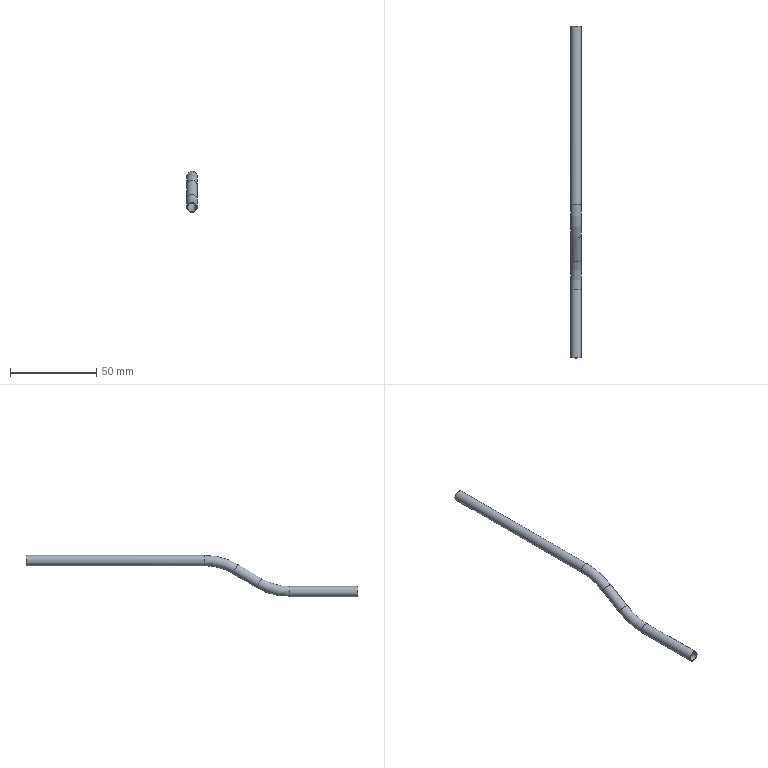Part | STEP file | 1-70.2 | 1 solid | 12 faces | box 6 x 192.5 x 24 mm | volume 1698 mm3 | cylinder 6 | torus 4 | plane 2 | commonest cylinder face diameters 5 x3 6 x3
STEP:
#1=CARTESIAN_POINT('',(0.,0.,0.));
#2=DIRECTION('',(0.,0.,1.));
#3=DIRECTION('',(1.,0.,0.));
#4=AXIS2_PLACEMENT_3D('',#1,#2,#3);
#5=CARTESIAN_POINT('',(-3.,103.5,0.));
#6=VERTEX_POINT('',#5);
#7=CARTESIAN_POINT('',(0.,103.5,0.));
#8=DIRECTION('',(0.,1.,0.));
#9=DIRECTION('',(-1.,0.,0.));
#10=AXIS2_PLACEMENT_3D('',#7,#8,#9);
#11=CIRCLE('',#10,3.);
#12=CARTESIAN_POINT('',(0.,103.5,0.));
#13=DIRECTION('',(0.,-1.,0.));
#14=DIRECTION('',(-1.,0.,0.));
#15=AXIS2_PLACEMENT_3D('',#12,#13,#14);
#16=CYLINDRICAL_SURFACE('',#15,3.);
#17=CARTESIAN_POINT('',(6.283,0.));
#18=DIRECTION('',(-1.,0.));
#19=VECTOR('',#18,1.);
#20=LINE('',#17,#19);
#21=(GEOMETRIC_REPRESENTATION_CONTEXT(2)PARAMETRIC_REPRESENTATION_CONTEXT()REPRESENTATION_CONTEXT('',''));
#22=DEFINITIONAL_REPRESENTATION('',(#20),#21);
#23=PCURVE('',#16,#22);
#24=CARTESIAN_POINT('',(0.,103.5,0.));
#25=DIRECTION('',(0.,1.,0.));
#26=DIRECTION('',(0.,0.,1.));
#27=AXIS2_PLACEMENT_3D('',#24,#25,#26);
#28=PLANE('',#27);
#29=CARTESIAN_POINT('',(0.,0.));
#30=DIRECTION('',(0.,-1.));
#31=AXIS2_PLACEMENT_2D('',#29,#30);
#32=CIRCLE('',#31,3.);
#33=(GEOMETRIC_REPRESENTATION_CONTEXT(2)PARAMETRIC_REPRESENTATION_CONTEXT()REPRESENTATION_CONTEXT('',''));
#34=DEFINITIONAL_REPRESENTATION('',(#32),#33);
#35=PCURVE('',#28,#34);
#36=SURFACE_CURVE('',#11,(#23,#35),.PCURVE_S1.);
#37=EDGE_CURVE('',#6,#6,#36,.T.);
#38=ORIENTED_EDGE('',*,*,#37,.F.);
#39=CARTESIAN_POINT('',(-3.,0.,0.));
#40=VERTEX_POINT('',#39);
#41=CARTESIAN_POINT('',(-3.,103.5,0.));
#42=DIRECTION('',(0.,-1.,0.));
#43=VECTOR('',#42,1.);
#44=LINE('',#41,#43);
#45=CARTESIAN_POINT('',(6.283,0.));
#46=DIRECTION('',(0.,1.));
#47=VECTOR('',#46,1.);
#48=LINE('',#45,#47);
#49=(GEOMETRIC_REPRESENTATION_CONTEXT(2)PARAMETRIC_REPRESENTATION_CONTEXT()REPRESENTATION_CONTEXT('',''));
#50=DEFINITIONAL_REPRESENTATION('',(#48),#49);
#51=PCURVE('',#16,#50);
#52=CARTESIAN_POINT('',(0.,0.));
#53=DIRECTION('',(0.,1.));
#54=VECTOR('',#53,1.);
#55=LINE('',#52,#54);
#56=(GEOMETRIC_REPRESENTATION_CONTEXT(2)PARAMETRIC_REPRESENTATION_CONTEXT()REPRESENTATION_CONTEXT('',''));
#57=DEFINITIONAL_REPRESENTATION('',(#55),#56);
#58=PCURVE('',#16,#57);
#59=SEAM_CURVE('',#44,(#51,#58),.PCURVE_S1.);
#60=EDGE_CURVE('',#6,#40,#59,.T.);
#61=ORIENTED_EDGE('',*,*,#60,.T.);
#62=CARTESIAN_POINT('',(0.,0.,-3.));
#63=VERTEX_POINT('',#62);
#64=CARTESIAN_POINT('',(0.,0.,0.));
#65=DIRECTION('',(0.,-1.,0.));
#66=DIRECTION('',(0.,0.,-1.));
#67=AXIS2_PLACEMENT_3D('',#64,#65,#66);
#68=CIRCLE('',#67,3.);
#69=CARTESIAN_POINT('',(1.571,103.5));
#70=DIRECTION('',(1.,0.));
#71=VECTOR('',#70,1.);
#72=LINE('',#69,#71);
#73=(GEOMETRIC_REPRESENTATION_CONTEXT(2)PARAMETRIC_REPRESENTATION_CONTEXT()REPRESENTATION_CONTEXT('',''));
#74=DEFINITIONAL_REPRESENTATION('',(#72),#73);
#75=PCURVE('',#16,#74);
#76=CARTESIAN_POINT('',(0.,0.,-35.));
#77=DIRECTION('',(-1.,0.,0.));
#78=DIRECTION('',(0.,0.,1.));
#79=AXIS2_PLACEMENT_3D('',#76,#77,#78);
#80=TOROIDAL_SURFACE('',#79,35.,3.);
#81=CARTESIAN_POINT('',(6.283,-3.142));
#82=DIRECTION('',(0.,1.));
#83=VECTOR('',#82,1.);
#84=LINE('',#81,#83);
#85=(GEOMETRIC_REPRESENTATION_CONTEXT(2)PARAMETRIC_REPRESENTATION_CONTEXT()REPRESENTATION_CONTEXT('',''));
#86=DEFINITIONAL_REPRESENTATION('',(#84),#85);
#87=PCURVE('',#80,#86);
#88=SURFACE_CURVE('',#68,(#75,#87),.PCURVE_S1.);
#89=EDGE_CURVE('',#63,#40,#88,.T.);
#90=ORIENTED_EDGE('',*,*,#89,.F.);
#91=CARTESIAN_POINT('',(0.,0.,0.));
#92=DIRECTION('',(0.,-1.,0.));
#93=DIRECTION('',(-1.,0.,0.));
#94=AXIS2_PLACEMENT_3D('',#91,#92,#93);
#95=CIRCLE('',#94,3.);
#96=CARTESIAN_POINT('',(0.,103.5));
#97=DIRECTION('',(1.,0.));
#98=VECTOR('',#97,1.);
#99=LINE('',#96,#98);
#100=(GEOMETRIC_REPRESENTATION_CONTEXT(2)PARAMETRIC_REPRESENTATION_CONTEXT()REPRESENTATION_CONTEXT('',''));
#101=DEFINITIONAL_REPRESENTATION('',(#99),#100);
#102=PCURVE('',#16,#101);
#103=CARTESIAN_POINT('',(6.283,1.571));
#104=DIRECTION('',(0.,1.));
#105=VECTOR('',#104,1.);
#106=LINE('',#103,#105);
#107=(GEOMETRIC_REPRESENTATION_CONTEXT(2)PARAMETRIC_REPRESENTATION_CONTEXT()REPRESENTATION_CONTEXT('',''));
#108=DEFINITIONAL_REPRESENTATION('',(#106),#107);
#109=PCURVE('',#80,#108);
#110=SURFACE_CURVE('',#95,(#102,#109),.PCURVE_S1.);
#111=EDGE_CURVE('',#40,#63,#110,.T.);
#112=ORIENTED_EDGE('',*,*,#111,.F.);
#113=ORIENTED_EDGE('',*,*,#60,.F.);
#114=EDGE_LOOP('',(#38,#61,#90,#112,#113));
#115=FACE_BOUND('',#114,.T.);
#116=ADVANCED_FACE('',(#115),#16,.T.);
#117=ORIENTED_EDGE('',*,*,#89,.T.);
#118=ORIENTED_EDGE('',*,*,#111,.T.);
#119=CARTESIAN_POINT('',(0.,-16.365,-7.501));
#120=VERTEX_POINT('',#119);
#121=CARTESIAN_POINT('',(0.,0.,-35.));
#122=DIRECTION('',(1.,0.,0.));
#123=DIRECTION('',(0.,0.,1.));
#124=AXIS2_PLACEMENT_3D('',#121,#122,#123);
#125=CIRCLE('',#124,32.);
#126=CARTESIAN_POINT('',(6.283,3.142));
#127=DIRECTION('',(-1.,0.));
#128=VECTOR('',#127,1.);
#129=LINE('',#126,#128);
#130=(GEOMETRIC_REPRESENTATION_CONTEXT(2)PARAMETRIC_REPRESENTATION_CONTEXT()REPRESENTATION_CONTEXT('',''));
#131=DEFINITIONAL_REPRESENTATION('',(#129),#130);
#132=PCURVE('',#80,#131);
#133=CARTESIAN_POINT('',(6.283,-3.142));
#134=DIRECTION('',(-1.,0.));
#135=VECTOR('',#134,1.);
#136=LINE('',#133,#135);
#137=(GEOMETRIC_REPRESENTATION_CONTEXT(2)PARAMETRIC_REPRESENTATION_CONTEXT()REPRESENTATION_CONTEXT('',''));
#138=DEFINITIONAL_REPRESENTATION('',(#136),#137);
#139=PCURVE('',#80,#138);
#140=SEAM_CURVE('',#125,(#132,#139),.PCURVE_S1.);
#141=EDGE_CURVE('',#63,#120,#140,.T.);
#142=ORIENTED_EDGE('',*,*,#141,.T.);
#143=CARTESIAN_POINT('',(-3.,-17.899,-4.923));
#144=VERTEX_POINT('',#143);
#145=CARTESIAN_POINT('',(0.,-17.899,-4.923));
#146=DIRECTION('',(0.,0.8593,0.5114));
#147=DIRECTION('',(0.,0.5114,-0.8593));
#148=AXIS2_PLACEMENT_3D('',#145,#146,#147);
#149=CIRCLE('',#148,3.);
#150=CARTESIAN_POINT('',(5.746,3.142));
#151=DIRECTION('',(0.,-1.));
#152=VECTOR('',#151,1.);
#153=LINE('',#150,#152);
#154=(GEOMETRIC_REPRESENTATION_CONTEXT(2)PARAMETRIC_REPRESENTATION_CONTEXT()REPRESENTATION_CONTEXT('',''));
#155=DEFINITIONAL_REPRESENTATION('',(#153),#154);
#156=PCURVE('',#80,#155);
#157=CARTESIAN_POINT('',(0.,-17.899,-4.923));
#158=DIRECTION('',(0.,-0.8593,-0.5114));
#159=DIRECTION('',(-1.,0.,0.));
#160=AXIS2_PLACEMENT_3D('',#157,#158,#159);
#161=CYLINDRICAL_SURFACE('',#160,3.);
#162=CARTESIAN_POINT('',(1.571,0.));
#163=DIRECTION('',(-1.,0.));
#164=VECTOR('',#163,1.);
#165=LINE('',#162,#164);
#166=(GEOMETRIC_REPRESENTATION_CONTEXT(2)PARAMETRIC_REPRESENTATION_CONTEXT()REPRESENTATION_CONTEXT('',''));
#167=DEFINITIONAL_REPRESENTATION('',(#165),#166);
#168=PCURVE('',#161,#167);
#169=SURFACE_CURVE('',#149,(#156,#168),.PCURVE_S1.);
#170=EDGE_CURVE('',#120,#144,#169,.T.);
#171=ORIENTED_EDGE('',*,*,#170,.T.);
#172=CARTESIAN_POINT('',(0.,-17.899,-4.923));
#173=DIRECTION('',(0.,0.8593,0.5114));
#174=DIRECTION('',(-1.,0.,0.));
#175=AXIS2_PLACEMENT_3D('',#172,#173,#174);
#176=CIRCLE('',#175,3.);
#177=CARTESIAN_POINT('',(5.746,1.571));
#178=DIRECTION('',(0.,-1.));
#179=VECTOR('',#178,1.);
#180=LINE('',#177,#179);
#181=(GEOMETRIC_REPRESENTATION_CONTEXT(2)PARAMETRIC_REPRESENTATION_CONTEXT()REPRESENTATION_CONTEXT('',''));
#182=DEFINITIONAL_REPRESENTATION('',(#180),#181);
#183=PCURVE('',#80,#182);
#184=CARTESIAN_POINT('',(6.283,0.));
#185=DIRECTION('',(-1.,0.));
#186=VECTOR('',#185,1.);
#187=LINE('',#184,#186);
#188=(GEOMETRIC_REPRESENTATION_CONTEXT(2)PARAMETRIC_REPRESENTATION_CONTEXT()REPRESENTATION_CONTEXT('',''));
#189=DEFINITIONAL_REPRESENTATION('',(#187),#188);
#190=PCURVE('',#161,#189);
#191=SURFACE_CURVE('',#176,(#183,#190),.PCURVE_S1.);
#192=EDGE_CURVE('',#144,#120,#191,.T.);
#193=ORIENTED_EDGE('',*,*,#192,.T.);
#194=ORIENTED_EDGE('',*,*,#141,.F.);
#195=EDGE_LOOP('',(#117,#118,#142,#171,#193,#194));
#196=FACE_BOUND('',#195,.T.);
#197=ADVANCED_FACE('',(#196),#80,.T.);
#198=ORIENTED_EDGE('',*,*,#170,.F.);
#199=ORIENTED_EDGE('',*,*,#192,.F.);
#200=CARTESIAN_POINT('',(-3.,-31.601,-13.077));
#201=VERTEX_POINT('',#200);
#202=CARTESIAN_POINT('',(-3.,-17.899,-4.923));
#203=DIRECTION('',(0.,-0.8593,-0.5114));
#204=VECTOR('',#203,1.);
#205=LINE('',#202,#204);
#206=CARTESIAN_POINT('',(6.283,0.));
#207=DIRECTION('',(0.,1.));
#208=VECTOR('',#207,1.);
#209=LINE('',#206,#208);
#210=(GEOMETRIC_REPRESENTATION_CONTEXT(2)PARAMETRIC_REPRESENTATION_CONTEXT()REPRESENTATION_CONTEXT('',''));
#211=DEFINITIONAL_REPRESENTATION('',(#209),#210);
#212=PCURVE('',#161,#211);
#213=CARTESIAN_POINT('',(0.,0.));
#214=DIRECTION('',(0.,1.));
#215=VECTOR('',#214,1.);
#216=LINE('',#213,#215);
#217=(GEOMETRIC_REPRESENTATION_CONTEXT(2)PARAMETRIC_REPRESENTATION_CONTEXT()REPRESENTATION_CONTEXT('',''));
#218=DEFINITIONAL_REPRESENTATION('',(#216),#217);
#219=PCURVE('',#161,#218);
#220=SEAM_CURVE('',#205,(#212,#219),.PCURVE_S1.);
#221=EDGE_CURVE('',#144,#201,#220,.T.);
#222=ORIENTED_EDGE('',*,*,#221,.T.);
#223=CARTESIAN_POINT('',(0.,-31.601,-13.077));
#224=DIRECTION('',(0.,-0.8593,-0.5114));
#225=DIRECTION('',(-1.,0.,0.));
#226=AXIS2_PLACEMENT_3D('',#223,#224,#225);
#227=CIRCLE('',#226,3.);
#228=CARTESIAN_POINT('',(0.,15.945));
#229=DIRECTION('',(1.,0.));
#230=VECTOR('',#229,1.);
#231=LINE('',#228,#230);
#232=(GEOMETRIC_REPRESENTATION_CONTEXT(2)PARAMETRIC_REPRESENTATION_CONTEXT()REPRESENTATION_CONTEXT('',''));
#233=DEFINITIONAL_REPRESENTATION('',(#231),#232);
#234=PCURVE('',#161,#233);
#235=CARTESIAN_POINT('',(0.,-49.5,17.));
#236=DIRECTION('',(1.,0.,0.));
#237=DIRECTION('',(0.,0.5114,-0.8593));
#238=AXIS2_PLACEMENT_3D('',#235,#236,#237);
#239=TOROIDAL_SURFACE('',#238,35.,3.);
#240=CARTESIAN_POINT('',(6.283,-1.571));
#241=DIRECTION('',(0.,1.));
#242=VECTOR('',#241,1.);
#243=LINE('',#240,#242);
#244=(GEOMETRIC_REPRESENTATION_CONTEXT(2)PARAMETRIC_REPRESENTATION_CONTEXT()REPRESENTATION_CONTEXT('',''));
#245=DEFINITIONAL_REPRESENTATION('',(#243),#244);
#246=PCURVE('',#239,#245);
#247=SURFACE_CURVE('',#227,(#234,#246),.PCURVE_S1.);
#248=EDGE_CURVE('',#201,#201,#247,.T.);
#249=ORIENTED_EDGE('',*,*,#248,.F.);
#250=ORIENTED_EDGE('',*,*,#221,.F.);
#251=EDGE_LOOP('',(#198,#199,#222,#249,#250));
#252=FACE_BOUND('',#251,.T.);
#253=ADVANCED_FACE('',(#252),#161,.T.);
#254=ORIENTED_EDGE('',*,*,#248,.T.);
#255=CARTESIAN_POINT('',(-3.,-49.5,-18.));
#256=VERTEX_POINT('',#255);
#257=CARTESIAN_POINT('',(-3.,-49.5,17.));
#258=DIRECTION('',(-1.,0.,0.));
#259=DIRECTION('',(0.,0.5114,-0.8593));
#260=AXIS2_PLACEMENT_3D('',#257,#258,#259);
#261=CIRCLE('',#260,35.);
#262=CARTESIAN_POINT('',(6.283,4.712));
#263=DIRECTION('',(-1.,0.));
#264=VECTOR('',#263,1.);
#265=LINE('',#262,#264);
#266=(GEOMETRIC_REPRESENTATION_CONTEXT(2)PARAMETRIC_REPRESENTATION_CONTEXT()REPRESENTATION_CONTEXT('',''));
#267=DEFINITIONAL_REPRESENTATION('',(#265),#266);
#268=PCURVE('',#239,#267);
#269=CARTESIAN_POINT('',(6.283,-1.571));
#270=DIRECTION('',(-1.,0.));
#271=VECTOR('',#270,1.);
#272=LINE('',#269,#271);
#273=(GEOMETRIC_REPRESENTATION_CONTEXT(2)PARAMETRIC_REPRESENTATION_CONTEXT()REPRESENTATION_CONTEXT('',''));
#274=DEFINITIONAL_REPRESENTATION('',(#272),#273);
#275=PCURVE('',#239,#274);
#276=SEAM_CURVE('',#261,(#268,#275),.PCURVE_S1.);
#277=EDGE_CURVE('',#201,#256,#276,.T.);
#278=ORIENTED_EDGE('',*,*,#277,.T.);
#279=CARTESIAN_POINT('',(0.,-49.5,-18.));
#280=DIRECTION('',(0.,1.,0.));
#281=DIRECTION('',(-1.,0.,0.));
#282=AXIS2_PLACEMENT_3D('',#279,#280,#281);
#283=CIRCLE('',#282,3.);
#284=CARTESIAN_POINT('',(5.746,4.712));
#285=DIRECTION('',(0.,-1.));
#286=VECTOR('',#285,1.);
#287=LINE('',#284,#286);
#288=(GEOMETRIC_REPRESENTATION_CONTEXT(2)PARAMETRIC_REPRESENTATION_CONTEXT()REPRESENTATION_CONTEXT('',''));
#289=DEFINITIONAL_REPRESENTATION('',(#287),#288);
#290=PCURVE('',#239,#289);
#291=CARTESIAN_POINT('',(0.,-49.5,-18.));
#292=DIRECTION('',(0.,-1.,0.));
#293=DIRECTION('',(-1.,0.,0.));
#294=AXIS2_PLACEMENT_3D('',#291,#292,#293);
#295=CYLINDRICAL_SURFACE('',#294,3.);
#296=CARTESIAN_POINT('',(6.283,0.));
#297=DIRECTION('',(-1.,0.));
#298=VECTOR('',#297,1.);
#299=LINE('',#296,#298);
#300=(GEOMETRIC_REPRESENTATION_CONTEXT(2)PARAMETRIC_REPRESENTATION_CONTEXT()REPRESENTATION_CONTEXT('',''));
#301=DEFINITIONAL_REPRESENTATION('',(#299),#300);
#302=PCURVE('',#295,#301);
#303=SURFACE_CURVE('',#283,(#290,#302),.PCURVE_S1.);
#304=EDGE_CURVE('',#256,#256,#303,.T.);
#305=ORIENTED_EDGE('',*,*,#304,.T.);
#306=ORIENTED_EDGE('',*,*,#277,.F.);
#307=EDGE_LOOP('',(#254,#278,#305,#306));
#308=FACE_BOUND('',#307,.T.);
#309=ADVANCED_FACE('',(#308),#239,.T.);
#310=ORIENTED_EDGE('',*,*,#304,.F.);
#311=CARTESIAN_POINT('',(-3.,-89.,-18.));
#312=VERTEX_POINT('',#311);
#313=CARTESIAN_POINT('',(-3.,-49.5,-18.));
#314=DIRECTION('',(0.,-1.,0.));
#315=VECTOR('',#314,1.);
#316=LINE('',#313,#315);
#317=CARTESIAN_POINT('',(6.283,0.));
#318=DIRECTION('',(0.,1.));
#319=VECTOR('',#318,1.);
#320=LINE('',#317,#319);
#321=(GEOMETRIC_REPRESENTATION_CONTEXT(2)PARAMETRIC_REPRESENTATION_CONTEXT()REPRESENTATION_CONTEXT('',''));
#322=DEFINITIONAL_REPRESENTATION('',(#320),#321);
#323=PCURVE('',#295,#322);
#324=CARTESIAN_POINT('',(0.,0.));
#325=DIRECTION('',(0.,1.));
#326=VECTOR('',#325,1.);
#327=LINE('',#324,#326);
#328=(GEOMETRIC_REPRESENTATION_CONTEXT(2)PARAMETRIC_REPRESENTATION_CONTEXT()REPRESENTATION_CONTEXT('',''));
#329=DEFINITIONAL_REPRESENTATION('',(#327),#328);
#330=PCURVE('',#295,#329);
#331=SEAM_CURVE('',#316,(#323,#330),.PCURVE_S1.);
#332=EDGE_CURVE('',#256,#312,#331,.T.);
#333=ORIENTED_EDGE('',*,*,#332,.T.);
#334=CARTESIAN_POINT('',(0.,-89.,-18.));
#335=DIRECTION('',(0.,-1.,0.));
#336=DIRECTION('',(-1.,0.,0.));
#337=AXIS2_PLACEMENT_3D('',#334,#335,#336);
#338=CIRCLE('',#337,3.);
#339=CARTESIAN_POINT('',(0.,39.5));
#340=DIRECTION('',(1.,0.));
#341=VECTOR('',#340,1.);
#342=LINE('',#339,#341);
#343=(GEOMETRIC_REPRESENTATION_CONTEXT(2)PARAMETRIC_REPRESENTATION_CONTEXT()REPRESENTATION_CONTEXT('',''));
#344=DEFINITIONAL_REPRESENTATION('',(#342),#343);
#345=PCURVE('',#295,#344);
#346=CARTESIAN_POINT('',(0.,-89.,-18.));
#347=DIRECTION('',(0.,-1.,0.));
#348=DIRECTION('',(0.,0.,-1.));
#349=AXIS2_PLACEMENT_3D('',#346,#347,#348);
#350=PLANE('',#349);
#351=CARTESIAN_POINT('',(0.,0.));
#352=DIRECTION('',(0.,-1.));
#353=AXIS2_PLACEMENT_2D('',#351,#352);
#354=CIRCLE('',#353,3.);
#355=(GEOMETRIC_REPRESENTATION_CONTEXT(2)PARAMETRIC_REPRESENTATION_CONTEXT()REPRESENTATION_CONTEXT('',''));
#356=DEFINITIONAL_REPRESENTATION('',(#354),#355);
#357=PCURVE('',#350,#356);
#358=SURFACE_CURVE('',#338,(#345,#357),.PCURVE_S1.);
#359=EDGE_CURVE('',#312,#312,#358,.T.);
#360=ORIENTED_EDGE('',*,*,#359,.F.);
#361=ORIENTED_EDGE('',*,*,#332,.F.);
#362=EDGE_LOOP('',(#310,#333,#360,#361));
#363=FACE_BOUND('',#362,.T.);
#364=ADVANCED_FACE('',(#363),#295,.T.);
#365=ORIENTED_EDGE('',*,*,#37,.T.);
#366=EDGE_LOOP('',(#365));
#367=FACE_BOUND('',#366,.T.);
#368=CARTESIAN_POINT('',(-2.5,103.5,0.));
#369=VERTEX_POINT('',#368);
#370=CARTESIAN_POINT('',(0.,103.5,0.));
#371=DIRECTION('',(0.,1.,0.));
#372=DIRECTION('',(-1.,0.,0.));
#373=AXIS2_PLACEMENT_3D('',#370,#371,#372);
#374=CIRCLE('',#373,2.5);
#375=CARTESIAN_POINT('',(0.,0.));
#376=DIRECTION('',(0.,-1.));
#377=AXIS2_PLACEMENT_2D('',#375,#376);
#378=CIRCLE('',#377,2.5);
#379=(GEOMETRIC_REPRESENTATION_CONTEXT(2)PARAMETRIC_REPRESENTATION_CONTEXT()REPRESENTATION_CONTEXT('',''));
#380=DEFINITIONAL_REPRESENTATION('',(#378),#379);
#381=PCURVE('',#28,#380);
#382=CARTESIAN_POINT('',(0.,103.5,0.));
#383=DIRECTION('',(0.,-1.,0.));
#384=DIRECTION('',(-1.,0.,0.));
#385=AXIS2_PLACEMENT_3D('',#382,#383,#384);
#386=CYLINDRICAL_SURFACE('',#385,2.5);
#387=CARTESIAN_POINT('',(6.283,0.));
#388=DIRECTION('',(-1.,0.));
#389=VECTOR('',#388,1.);
#390=LINE('',#387,#389);
#391=(GEOMETRIC_REPRESENTATION_CONTEXT(2)PARAMETRIC_REPRESENTATION_CONTEXT()REPRESENTATION_CONTEXT('',''));
#392=DEFINITIONAL_REPRESENTATION('',(#390),#391);
#393=PCURVE('',#386,#392);
#394=SURFACE_CURVE('',#374,(#381,#393),.PCURVE_S1.);
#395=EDGE_CURVE('',#369,#369,#394,.T.);
#396=ORIENTED_EDGE('',*,*,#395,.F.);
#397=EDGE_LOOP('',(#396));
#398=FACE_BOUND('',#397,.T.);
#399=ADVANCED_FACE('',(#367,#398),#28,.T.);
#400=ORIENTED_EDGE('',*,*,#359,.T.);
#401=EDGE_LOOP('',(#400));
#402=FACE_BOUND('',#401,.T.);
#403=CARTESIAN_POINT('',(-2.5,-89.,-18.));
#404=VERTEX_POINT('',#403);
#405=CARTESIAN_POINT('',(0.,-89.,-18.));
#406=DIRECTION('',(0.,-1.,0.));
#407=DIRECTION('',(-1.,0.,0.));
#408=AXIS2_PLACEMENT_3D('',#405,#406,#407);
#409=CIRCLE('',#408,2.5);
#410=CARTESIAN_POINT('',(0.,0.));
#411=DIRECTION('',(0.,-1.));
#412=AXIS2_PLACEMENT_2D('',#410,#411);
#413=CIRCLE('',#412,2.5);
#414=(GEOMETRIC_REPRESENTATION_CONTEXT(2)PARAMETRIC_REPRESENTATION_CONTEXT()REPRESENTATION_CONTEXT('',''));
#415=DEFINITIONAL_REPRESENTATION('',(#413),#414);
#416=PCURVE('',#350,#415);
#417=CARTESIAN_POINT('',(0.,-49.5,-18.));
#418=DIRECTION('',(0.,-1.,0.));
#419=DIRECTION('',(-1.,0.,0.));
#420=AXIS2_PLACEMENT_3D('',#417,#418,#419);
#421=CYLINDRICAL_SURFACE('',#420,2.5);
#422=CARTESIAN_POINT('',(0.,39.5));
#423=DIRECTION('',(1.,0.));
#424=VECTOR('',#423,1.);
#425=LINE('',#422,#424);
#426=(GEOMETRIC_REPRESENTATION_CONTEXT(2)PARAMETRIC_REPRESENTATION_CONTEXT()REPRESENTATION_CONTEXT('',''));
#427=DEFINITIONAL_REPRESENTATION('',(#425),#426);
#428=PCURVE('',#421,#427);
#429=SURFACE_CURVE('',#409,(#416,#428),.PCURVE_S1.);
#430=EDGE_CURVE('',#404,#404,#429,.T.);
#431=ORIENTED_EDGE('',*,*,#430,.F.);
#432=EDGE_LOOP('',(#431));
#433=FACE_BOUND('',#432,.T.);
#434=ADVANCED_FACE('',(#402,#433),#350,.T.);
#435=ORIENTED_EDGE('',*,*,#395,.F.);
#436=CARTESIAN_POINT('',(-2.5,0.,0.));
#437=VERTEX_POINT('',#436);
#438=CARTESIAN_POINT('',(-2.5,103.5,0.));
#439=DIRECTION('',(0.,-1.,0.));
#440=VECTOR('',#439,1.);
#441=LINE('',#438,#440);
#442=CARTESIAN_POINT('',(6.283,0.));
#443=DIRECTION('',(0.,1.));
#444=VECTOR('',#443,1.);
#445=LINE('',#442,#444);
#446=(GEOMETRIC_REPRESENTATION_CONTEXT(2)PARAMETRIC_REPRESENTATION_CONTEXT()REPRESENTATION_CONTEXT('',''));
#447=DEFINITIONAL_REPRESENTATION('',(#445),#446);
#448=PCURVE('',#386,#447);
#449=CARTESIAN_POINT('',(0.,0.));
#450=DIRECTION('',(0.,1.));
#451=VECTOR('',#450,1.);
#452=LINE('',#449,#451);
#453=(GEOMETRIC_REPRESENTATION_CONTEXT(2)PARAMETRIC_REPRESENTATION_CONTEXT()REPRESENTATION_CONTEXT('',''));
#454=DEFINITIONAL_REPRESENTATION('',(#452),#453);
#455=PCURVE('',#386,#454);
#456=SEAM_CURVE('',#441,(#448,#455),.PCURVE_S1.);
#457=EDGE_CURVE('',#369,#437,#456,.T.);
#458=ORIENTED_EDGE('',*,*,#457,.T.);
#459=CARTESIAN_POINT('',(0.,0.,-2.5));
#460=VERTEX_POINT('',#459);
#461=CARTESIAN_POINT('',(0.,0.,0.));
#462=DIRECTION('',(0.,-1.,0.));
#463=DIRECTION('',(0.,0.,-1.));
#464=AXIS2_PLACEMENT_3D('',#461,#462,#463);
#465=CIRCLE('',#464,2.5);
#466=CARTESIAN_POINT('',(1.571,103.5));
#467=DIRECTION('',(1.,0.));
#468=VECTOR('',#467,1.);
#469=LINE('',#466,#468);
#470=(GEOMETRIC_REPRESENTATION_CONTEXT(2)PARAMETRIC_REPRESENTATION_CONTEXT()REPRESENTATION_CONTEXT('',''));
#471=DEFINITIONAL_REPRESENTATION('',(#469),#470);
#472=PCURVE('',#386,#471);
#473=CARTESIAN_POINT('',(0.,0.,-35.));
#474=DIRECTION('',(-1.,0.,0.));
#475=DIRECTION('',(0.,0.,1.));
#476=AXIS2_PLACEMENT_3D('',#473,#474,#475);
#477=TOROIDAL_SURFACE('',#476,35.,2.5);
#478=CARTESIAN_POINT('',(6.283,3.142));
#479=DIRECTION('',(0.,1.));
#480=VECTOR('',#479,1.);
#481=LINE('',#478,#480);
#482=(GEOMETRIC_REPRESENTATION_CONTEXT(2)PARAMETRIC_REPRESENTATION_CONTEXT()REPRESENTATION_CONTEXT('',''));
#483=DEFINITIONAL_REPRESENTATION('',(#481),#482);
#484=PCURVE('',#477,#483);
#485=SURFACE_CURVE('',#465,(#472,#484),.PCURVE_S1.);
#486=EDGE_CURVE('',#460,#437,#485,.T.);
#487=ORIENTED_EDGE('',*,*,#486,.F.);
#488=CARTESIAN_POINT('',(0.,0.,0.));
#489=DIRECTION('',(0.,-1.,0.));
#490=DIRECTION('',(-1.,0.,0.));
#491=AXIS2_PLACEMENT_3D('',#488,#489,#490);
#492=CIRCLE('',#491,2.5);
#493=CARTESIAN_POINT('',(0.,103.5));
#494=DIRECTION('',(1.,0.));
#495=VECTOR('',#494,1.);
#496=LINE('',#493,#495);
#497=(GEOMETRIC_REPRESENTATION_CONTEXT(2)PARAMETRIC_REPRESENTATION_CONTEXT()REPRESENTATION_CONTEXT('',''));
#498=DEFINITIONAL_REPRESENTATION('',(#496),#497);
#499=PCURVE('',#386,#498);
#500=CARTESIAN_POINT('',(6.283,7.854));
#501=DIRECTION('',(0.,1.));
#502=VECTOR('',#501,1.);
#503=LINE('',#500,#502);
#504=(GEOMETRIC_REPRESENTATION_CONTEXT(2)PARAMETRIC_REPRESENTATION_CONTEXT()REPRESENTATION_CONTEXT('',''));
#505=DEFINITIONAL_REPRESENTATION('',(#503),#504);
#506=PCURVE('',#477,#505);
#507=SURFACE_CURVE('',#492,(#499,#506),.PCURVE_S1.);
#508=EDGE_CURVE('',#437,#460,#507,.T.);
#509=ORIENTED_EDGE('',*,*,#508,.F.);
#510=ORIENTED_EDGE('',*,*,#457,.F.);
#511=EDGE_LOOP('',(#435,#458,#487,#509,#510));
#512=FACE_BOUND('',#511,.F.);
#513=ADVANCED_FACE('',(#512),#386,.F.);
#514=ORIENTED_EDGE('',*,*,#486,.T.);
#515=ORIENTED_EDGE('',*,*,#508,.T.);
#516=CARTESIAN_POINT('',(0.,-16.62,-7.071));
#517=VERTEX_POINT('',#516);
#518=CARTESIAN_POINT('',(0.,0.,-35.));
#519=DIRECTION('',(1.,0.,0.));
#520=DIRECTION('',(0.,0.,1.));
#521=AXIS2_PLACEMENT_3D('',#518,#519,#520);
#522=CIRCLE('',#521,32.5);
#523=CARTESIAN_POINT('',(6.283,9.425));
#524=DIRECTION('',(-1.,0.));
#525=VECTOR('',#524,1.);
#526=LINE('',#523,#525);
#527=(GEOMETRIC_REPRESENTATION_CONTEXT(2)PARAMETRIC_REPRESENTATION_CONTEXT()REPRESENTATION_CONTEXT('',''));
#528=DEFINITIONAL_REPRESENTATION('',(#526),#527);
#529=PCURVE('',#477,#528);
#530=CARTESIAN_POINT('',(6.283,3.142));
#531=DIRECTION('',(-1.,0.));
#532=VECTOR('',#531,1.);
#533=LINE('',#530,#532);
#534=(GEOMETRIC_REPRESENTATION_CONTEXT(2)PARAMETRIC_REPRESENTATION_CONTEXT()REPRESENTATION_CONTEXT('',''));
#535=DEFINITIONAL_REPRESENTATION('',(#533),#534);
#536=PCURVE('',#477,#535);
#537=SEAM_CURVE('',#522,(#529,#536),.PCURVE_S1.);
#538=EDGE_CURVE('',#460,#517,#537,.T.);
#539=ORIENTED_EDGE('',*,*,#538,.T.);
#540=CARTESIAN_POINT('',(-2.5,-17.899,-4.923));
#541=VERTEX_POINT('',#540);
#542=CARTESIAN_POINT('',(0.,-17.899,-4.923));
#543=DIRECTION('',(0.,0.8593,0.5114));
#544=DIRECTION('',(0.,0.5114,-0.8593));
#545=AXIS2_PLACEMENT_3D('',#542,#543,#544);
#546=CIRCLE('',#545,2.5);
#547=CARTESIAN_POINT('',(5.746,9.425));
#548=DIRECTION('',(0.,-1.));
#549=VECTOR('',#548,1.);
#550=LINE('',#547,#549);
#551=(GEOMETRIC_REPRESENTATION_CONTEXT(2)PARAMETRIC_REPRESENTATION_CONTEXT()REPRESENTATION_CONTEXT('',''));
#552=DEFINITIONAL_REPRESENTATION('',(#550),#551);
#553=PCURVE('',#477,#552);
#554=CARTESIAN_POINT('',(0.,-17.899,-4.923));
#555=DIRECTION('',(0.,-0.8593,-0.5114));
#556=DIRECTION('',(-1.,0.,0.));
#557=AXIS2_PLACEMENT_3D('',#554,#555,#556);
#558=CYLINDRICAL_SURFACE('',#557,2.5);
#559=CARTESIAN_POINT('',(1.571,0.));
#560=DIRECTION('',(-1.,0.));
#561=VECTOR('',#560,1.);
#562=LINE('',#559,#561);
#563=(GEOMETRIC_REPRESENTATION_CONTEXT(2)PARAMETRIC_REPRESENTATION_CONTEXT()REPRESENTATION_CONTEXT('',''));
#564=DEFINITIONAL_REPRESENTATION('',(#562),#563);
#565=PCURVE('',#558,#564);
#566=SURFACE_CURVE('',#546,(#553,#565),.PCURVE_S1.);
#567=EDGE_CURVE('',#517,#541,#566,.T.);
#568=ORIENTED_EDGE('',*,*,#567,.T.);
#569=CARTESIAN_POINT('',(0.,-17.899,-4.923));
#570=DIRECTION('',(0.,0.8593,0.5114));
#571=DIRECTION('',(-1.,0.,0.));
#572=AXIS2_PLACEMENT_3D('',#569,#570,#571);
#573=CIRCLE('',#572,2.5);
#574=CARTESIAN_POINT('',(5.746,7.854));
#575=DIRECTION('',(0.,-1.));
#576=VECTOR('',#575,1.);
#577=LINE('',#574,#576);
#578=(GEOMETRIC_REPRESENTATION_CONTEXT(2)PARAMETRIC_REPRESENTATION_CONTEXT()REPRESENTATION_CONTEXT('',''));
#579=DEFINITIONAL_REPRESENTATION('',(#577),#578);
#580=PCURVE('',#477,#579);
#581=CARTESIAN_POINT('',(6.283,0.));
#582=DIRECTION('',(-1.,0.));
#583=VECTOR('',#582,1.);
#584=LINE('',#581,#583);
#585=(GEOMETRIC_REPRESENTATION_CONTEXT(2)PARAMETRIC_REPRESENTATION_CONTEXT()REPRESENTATION_CONTEXT('',''));
#586=DEFINITIONAL_REPRESENTATION('',(#584),#585);
#587=PCURVE('',#558,#586);
#588=SURFACE_CURVE('',#573,(#580,#587),.PCURVE_S1.);
#589=EDGE_CURVE('',#541,#517,#588,.T.);
#590=ORIENTED_EDGE('',*,*,#589,.T.);
#591=ORIENTED_EDGE('',*,*,#538,.F.);
#592=EDGE_LOOP('',(#514,#515,#539,#568,#590,#591));
#593=FACE_BOUND('',#592,.F.);
#594=ADVANCED_FACE('',(#593),#477,.F.);
#595=ORIENTED_EDGE('',*,*,#567,.F.);
#596=ORIENTED_EDGE('',*,*,#589,.F.);
#597=CARTESIAN_POINT('',(-2.5,-31.601,-13.077));
#598=VERTEX_POINT('',#597);
#599=CARTESIAN_POINT('',(-2.5,-17.899,-4.923));
#600=DIRECTION('',(0.,-0.8593,-0.5114));
#601=VECTOR('',#600,1.);
#602=LINE('',#599,#601);
#603=CARTESIAN_POINT('',(6.283,0.));
#604=DIRECTION('',(0.,1.));
#605=VECTOR('',#604,1.);
#606=LINE('',#603,#605);
#607=(GEOMETRIC_REPRESENTATION_CONTEXT(2)PARAMETRIC_REPRESENTATION_CONTEXT()REPRESENTATION_CONTEXT('',''));
#608=DEFINITIONAL_REPRESENTATION('',(#606),#607);
#609=PCURVE('',#558,#608);
#610=CARTESIAN_POINT('',(0.,0.));
#611=DIRECTION('',(0.,1.));
#612=VECTOR('',#611,1.);
#613=LINE('',#610,#612);
#614=(GEOMETRIC_REPRESENTATION_CONTEXT(2)PARAMETRIC_REPRESENTATION_CONTEXT()REPRESENTATION_CONTEXT('',''));
#615=DEFINITIONAL_REPRESENTATION('',(#613),#614);
#616=PCURVE('',#558,#615);
#617=SEAM_CURVE('',#602,(#609,#616),.PCURVE_S1.);
#618=EDGE_CURVE('',#541,#598,#617,.T.);
#619=ORIENTED_EDGE('',*,*,#618,.T.);
#620=CARTESIAN_POINT('',(0.,-31.601,-13.077));
#621=DIRECTION('',(0.,-0.8593,-0.5114));
#622=DIRECTION('',(-1.,0.,0.));
#623=AXIS2_PLACEMENT_3D('',#620,#621,#622);
#624=CIRCLE('',#623,2.5);
#625=CARTESIAN_POINT('',(0.,15.945));
#626=DIRECTION('',(1.,0.));
#627=VECTOR('',#626,1.);
#628=LINE('',#625,#627);
#629=(GEOMETRIC_REPRESENTATION_CONTEXT(2)PARAMETRIC_REPRESENTATION_CONTEXT()REPRESENTATION_CONTEXT('',''));
#630=DEFINITIONAL_REPRESENTATION('',(#628),#629);
#631=PCURVE('',#558,#630);
#632=CARTESIAN_POINT('',(0.,-49.5,17.));
#633=DIRECTION('',(1.,0.,0.));
#634=DIRECTION('',(0.,0.5114,-0.8593));
#635=AXIS2_PLACEMENT_3D('',#632,#633,#634);
#636=TOROIDAL_SURFACE('',#635,35.,2.5);
#637=CARTESIAN_POINT('',(6.283,-1.571));
#638=DIRECTION('',(0.,1.));
#639=VECTOR('',#638,1.);
#640=LINE('',#637,#639);
#641=(GEOMETRIC_REPRESENTATION_CONTEXT(2)PARAMETRIC_REPRESENTATION_CONTEXT()REPRESENTATION_CONTEXT('',''));
#642=DEFINITIONAL_REPRESENTATION('',(#640),#641);
#643=PCURVE('',#636,#642);
#644=SURFACE_CURVE('',#624,(#631,#643),.PCURVE_S1.);
#645=EDGE_CURVE('',#598,#598,#644,.T.);
#646=ORIENTED_EDGE('',*,*,#645,.F.);
#647=ORIENTED_EDGE('',*,*,#618,.F.);
#648=EDGE_LOOP('',(#595,#596,#619,#646,#647));
#649=FACE_BOUND('',#648,.F.);
#650=ADVANCED_FACE('',(#649),#558,.F.);
#651=ORIENTED_EDGE('',*,*,#645,.T.);
#652=CARTESIAN_POINT('',(-2.5,-49.5,-18.));
#653=VERTEX_POINT('',#652);
#654=CARTESIAN_POINT('',(-2.5,-49.5,17.));
#655=DIRECTION('',(-1.,0.,0.));
#656=DIRECTION('',(0.,0.5114,-0.8593));
#657=AXIS2_PLACEMENT_3D('',#654,#655,#656);
#658=CIRCLE('',#657,35.);
#659=CARTESIAN_POINT('',(6.283,4.712));
#660=DIRECTION('',(-1.,0.));
#661=VECTOR('',#660,1.);
#662=LINE('',#659,#661);
#663=(GEOMETRIC_REPRESENTATION_CONTEXT(2)PARAMETRIC_REPRESENTATION_CONTEXT()REPRESENTATION_CONTEXT('',''));
#664=DEFINITIONAL_REPRESENTATION('',(#662),#663);
#665=PCURVE('',#636,#664);
#666=CARTESIAN_POINT('',(6.283,-1.571));
#667=DIRECTION('',(-1.,0.));
#668=VECTOR('',#667,1.);
#669=LINE('',#666,#668);
#670=(GEOMETRIC_REPRESENTATION_CONTEXT(2)PARAMETRIC_REPRESENTATION_CONTEXT()REPRESENTATION_CONTEXT('',''));
#671=DEFINITIONAL_REPRESENTATION('',(#669),#670);
#672=PCURVE('',#636,#671);
#673=SEAM_CURVE('',#658,(#665,#672),.PCURVE_S1.);
#674=EDGE_CURVE('',#598,#653,#673,.T.);
#675=ORIENTED_EDGE('',*,*,#674,.T.);
#676=CARTESIAN_POINT('',(0.,-49.5,-18.));
#677=DIRECTION('',(0.,1.,0.));
#678=DIRECTION('',(-1.,0.,0.));
#679=AXIS2_PLACEMENT_3D('',#676,#677,#678);
#680=CIRCLE('',#679,2.5);
#681=CARTESIAN_POINT('',(5.746,4.712));
#682=DIRECTION('',(0.,-1.));
#683=VECTOR('',#682,1.);
#684=LINE('',#681,#683);
#685=(GEOMETRIC_REPRESENTATION_CONTEXT(2)PARAMETRIC_REPRESENTATION_CONTEXT()REPRESENTATION_CONTEXT('',''));
#686=DEFINITIONAL_REPRESENTATION('',(#684),#685);
#687=PCURVE('',#636,#686);
#688=CARTESIAN_POINT('',(6.283,0.));
#689=DIRECTION('',(-1.,0.));
#690=VECTOR('',#689,1.);
#691=LINE('',#688,#690);
#692=(GEOMETRIC_REPRESENTATION_CONTEXT(2)PARAMETRIC_REPRESENTATION_CONTEXT()REPRESENTATION_CONTEXT('',''));
#693=DEFINITIONAL_REPRESENTATION('',(#691),#692);
#694=PCURVE('',#421,#693);
#695=SURFACE_CURVE('',#680,(#687,#694),.PCURVE_S1.);
#696=EDGE_CURVE('',#653,#653,#695,.T.);
#697=ORIENTED_EDGE('',*,*,#696,.T.);
#698=ORIENTED_EDGE('',*,*,#674,.F.);
#699=EDGE_LOOP('',(#651,#675,#697,#698));
#700=FACE_BOUND('',#699,.F.);
#701=ADVANCED_FACE('',(#700),#636,.F.);
#702=ORIENTED_EDGE('',*,*,#696,.F.);
#703=CARTESIAN_POINT('',(-2.5,-49.5,-18.));
#704=DIRECTION('',(0.,-1.,0.));
#705=VECTOR('',#704,1.);
#706=LINE('',#703,#705);
#707=CARTESIAN_POINT('',(6.283,0.));
#708=DIRECTION('',(0.,1.));
#709=VECTOR('',#708,1.);
#710=LINE('',#707,#709);
#711=(GEOMETRIC_REPRESENTATION_CONTEXT(2)PARAMETRIC_REPRESENTATION_CONTEXT()REPRESENTATION_CONTEXT('',''));
#712=DEFINITIONAL_REPRESENTATION('',(#710),#711);
#713=PCURVE('',#421,#712);
#714=CARTESIAN_POINT('',(0.,0.));
#715=DIRECTION('',(0.,1.));
#716=VECTOR('',#715,1.);
#717=LINE('',#714,#716);
#718=(GEOMETRIC_REPRESENTATION_CONTEXT(2)PARAMETRIC_REPRESENTATION_CONTEXT()REPRESENTATION_CONTEXT('',''));
#719=DEFINITIONAL_REPRESENTATION('',(#717),#718);
#720=PCURVE('',#421,#719);
#721=SEAM_CURVE('',#706,(#713,#720),.PCURVE_S1.);
#722=EDGE_CURVE('',#653,#404,#721,.T.);
#723=ORIENTED_EDGE('',*,*,#722,.T.);
#724=ORIENTED_EDGE('',*,*,#430,.F.);
#725=ORIENTED_EDGE('',*,*,#722,.F.);
#726=EDGE_LOOP('',(#702,#723,#724,#725));
#727=FACE_BOUND('',#726,.F.);
#728=ADVANCED_FACE('',(#727),#421,.F.);
#729=CLOSED_SHELL('',(#116,#197,#253,#309,#364,#399,#434,#513,#594,#650,#701,#728));
#730=MANIFOLD_SOLID_BREP('',#729);
#731=(LENGTH_UNIT()NAMED_UNIT(*)SI_UNIT(.MILLI.,.METRE.));
#732=UNCERTAINTY_MEASURE_WITH_UNIT(LENGTH_MEASURE(0.0000001),#731,'','');
#733=(NAMED_UNIT(*)PLANE_ANGLE_UNIT()SI_UNIT($,.RADIAN.));
#734=(NAMED_UNIT(*)SI_UNIT($,.STERADIAN.)SOLID_ANGLE_UNIT());
#735=(GEOMETRIC_REPRESENTATION_CONTEXT(3)GLOBAL_UNCERTAINTY_ASSIGNED_CONTEXT((#732))GLOBAL_UNIT_ASSIGNED_CONTEXT((#731,#733,#734))REPRESENTATION_CONTEXT('',''));
#736=ADVANCED_BREP_SHAPE_REPRESENTATION('',(#4,#730),#735);